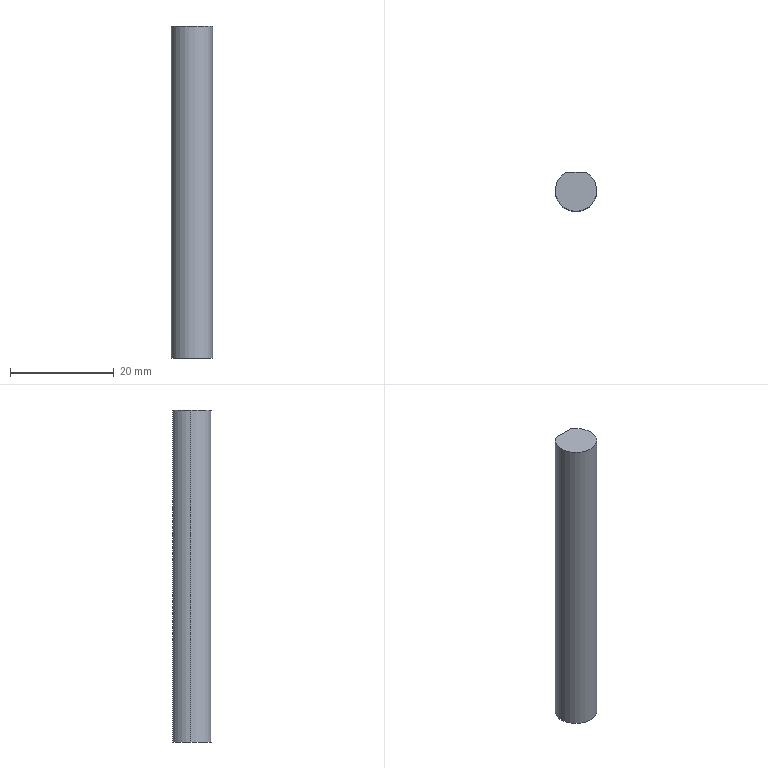Part | NX | features BREP 1 | 1 solid | 6 faces | box 8 x 7.5 x 64 mm | volume 3133 mm3 | cylinder 3 | plane 3 | commonest cylinder face diameters 8 x3
STEP:
#1=CARTESIAN_POINT('',(1.936,3.5,63.));
#2=VERTEX_POINT('',#1);
#3=CARTESIAN_POINT('',(4.,0.,63.));
#4=VERTEX_POINT('',#3);
#5=CARTESIAN_POINT('',(0.,0.,63.));
#6=DIRECTION('',(0.,0.,-1.));
#7=DIRECTION('',(-1.,0.,0.));
#8=AXIS2_PLACEMENT_3D('',#5,#6,#7);
#9=CIRCLE('',#8,4.);
#10=EDGE_CURVE('',#2,#4,#9,.T.);
#11=ORIENTED_EDGE('',*,*,#10,.T.);
#12=CARTESIAN_POINT('',(4.,0.,-1.));
#13=VERTEX_POINT('',#12);
#14=CARTESIAN_POINT('',(4.,0.,63.));
#15=DIRECTION('',(0.,0.,-1.));
#16=VECTOR('',#15,1000.);
#17=LINE('',#14,#16);
#18=EDGE_CURVE('',#4,#13,#17,.T.);
#19=ORIENTED_EDGE('',*,*,#18,.T.);
#20=CARTESIAN_POINT('',(1.936,3.5,-1.));
#21=VERTEX_POINT('',#20);
#22=CARTESIAN_POINT('',(0.,0.,-1.));
#23=DIRECTION('',(0.,0.,1.));
#24=DIRECTION('',(-1.,0.,0.));
#25=AXIS2_PLACEMENT_3D('',#22,#23,#24);
#26=CIRCLE('',#25,4.);
#27=EDGE_CURVE('',#13,#21,#26,.T.);
#28=ORIENTED_EDGE('',*,*,#27,.T.);
#29=CARTESIAN_POINT('',(1.936,3.5,63.));
#30=DIRECTION('',(0.,0.,1.));
#31=VECTOR('',#30,1000.);
#32=LINE('',#29,#31);
#33=EDGE_CURVE('',#21,#2,#32,.T.);
#34=ORIENTED_EDGE('',*,*,#33,.T.);
#35=EDGE_LOOP('',(#11,#19,#28,#34));
#36=FACE_BOUND('',#35,.T.);
#37=CARTESIAN_POINT('',(0.,0.,63.));
#38=DIRECTION('',(0.,0.,-1.));
#39=DIRECTION('',(-1.,0.,0.));
#40=AXIS2_PLACEMENT_3D('',#37,#38,#39);
#41=CYLINDRICAL_SURFACE('',#40,4.);
#42=ADVANCED_FACE('',(#36),#41,.T.);
#43=ORIENTED_EDGE('',*,*,#18,.F.);
#44=CARTESIAN_POINT('',(-4.,0.,63.));
#45=VERTEX_POINT('',#44);
#46=CARTESIAN_POINT('',(0.,0.,63.));
#47=DIRECTION('',(0.,0.,-1.));
#48=DIRECTION('',(-1.,0.,0.));
#49=AXIS2_PLACEMENT_3D('',#46,#47,#48);
#50=CIRCLE('',#49,4.);
#51=EDGE_CURVE('',#4,#45,#50,.T.);
#52=ORIENTED_EDGE('',*,*,#51,.T.);
#53=CARTESIAN_POINT('',(-4.,0.,-1.));
#54=VERTEX_POINT('',#53);
#55=CARTESIAN_POINT('',(-4.,0.,63.));
#56=DIRECTION('',(0.,0.,-1.));
#57=VECTOR('',#56,1000.);
#58=LINE('',#55,#57);
#59=EDGE_CURVE('',#45,#54,#58,.T.);
#60=ORIENTED_EDGE('',*,*,#59,.T.);
#61=CARTESIAN_POINT('',(0.,0.,-1.));
#62=DIRECTION('',(0.,0.,1.));
#63=DIRECTION('',(-1.,0.,0.));
#64=AXIS2_PLACEMENT_3D('',#61,#62,#63);
#65=CIRCLE('',#64,4.);
#66=EDGE_CURVE('',#54,#13,#65,.T.);
#67=ORIENTED_EDGE('',*,*,#66,.T.);
#68=EDGE_LOOP('',(#43,#52,#60,#67));
#69=FACE_BOUND('',#68,.T.);
#70=CARTESIAN_POINT('',(0.,0.,63.));
#71=DIRECTION('',(0.,0.,-1.));
#72=DIRECTION('',(-1.,0.,0.));
#73=AXIS2_PLACEMENT_3D('',#70,#71,#72);
#74=CYLINDRICAL_SURFACE('',#73,4.);
#75=ADVANCED_FACE('',(#69),#74,.T.);
#76=ORIENTED_EDGE('',*,*,#59,.F.);
#77=CARTESIAN_POINT('',(-1.936,3.5,63.));
#78=VERTEX_POINT('',#77);
#79=CARTESIAN_POINT('',(0.,0.,63.));
#80=DIRECTION('',(0.,0.,-1.));
#81=DIRECTION('',(-1.,0.,0.));
#82=AXIS2_PLACEMENT_3D('',#79,#80,#81);
#83=CIRCLE('',#82,4.);
#84=EDGE_CURVE('',#45,#78,#83,.T.);
#85=ORIENTED_EDGE('',*,*,#84,.T.);
#86=CARTESIAN_POINT('',(-1.936,3.5,-1.));
#87=VERTEX_POINT('',#86);
#88=CARTESIAN_POINT('',(-1.936,3.5,63.));
#89=DIRECTION('',(0.,0.,-1.));
#90=VECTOR('',#89,1000.);
#91=LINE('',#88,#90);
#92=EDGE_CURVE('',#78,#87,#91,.T.);
#93=ORIENTED_EDGE('',*,*,#92,.T.);
#94=CARTESIAN_POINT('',(0.,0.,-1.));
#95=DIRECTION('',(0.,0.,1.));
#96=DIRECTION('',(-1.,0.,0.));
#97=AXIS2_PLACEMENT_3D('',#94,#95,#96);
#98=CIRCLE('',#97,4.);
#99=EDGE_CURVE('',#87,#54,#98,.T.);
#100=ORIENTED_EDGE('',*,*,#99,.T.);
#101=EDGE_LOOP('',(#76,#85,#93,#100));
#102=FACE_BOUND('',#101,.T.);
#103=CARTESIAN_POINT('',(0.,0.,63.));
#104=DIRECTION('',(0.,0.,-1.));
#105=DIRECTION('',(-1.,0.,0.));
#106=AXIS2_PLACEMENT_3D('',#103,#104,#105);
#107=CYLINDRICAL_SURFACE('',#106,4.);
#108=ADVANCED_FACE('',(#102),#107,.T.);
#109=CARTESIAN_POINT('',(0.,3.5,-1.));
#110=DIRECTION('',(-1.,0.,0.));
#111=VECTOR('',#110,1000.);
#112=LINE('',#109,#111);
#113=EDGE_CURVE('',#21,#87,#112,.T.);
#114=ORIENTED_EDGE('',*,*,#113,.F.);
#115=ORIENTED_EDGE('',*,*,#27,.F.);
#116=ORIENTED_EDGE('',*,*,#66,.F.);
#117=ORIENTED_EDGE('',*,*,#99,.F.);
#118=EDGE_LOOP('',(#114,#115,#116,#117));
#119=FACE_BOUND('',#118,.T.);
#120=CARTESIAN_POINT('',(0.,0.,-1.));
#121=DIRECTION('',(0.,0.,1.));
#122=DIRECTION('',(1.,0.,0.));
#123=AXIS2_PLACEMENT_3D('',#120,#121,#122);
#124=PLANE('',#123);
#125=ADVANCED_FACE('',(#119),#124,.F.);
#126=ORIENTED_EDGE('',*,*,#10,.F.);
#127=CARTESIAN_POINT('',(0.,3.5,63.));
#128=DIRECTION('',(-1.,0.,0.));
#129=VECTOR('',#128,1000.);
#130=LINE('',#127,#129);
#131=EDGE_CURVE('',#2,#78,#130,.T.);
#132=ORIENTED_EDGE('',*,*,#131,.T.);
#133=ORIENTED_EDGE('',*,*,#84,.F.);
#134=ORIENTED_EDGE('',*,*,#51,.F.);
#135=EDGE_LOOP('',(#126,#132,#133,#134));
#136=FACE_BOUND('',#135,.T.);
#137=CARTESIAN_POINT('',(0.,0.,63.));
#138=DIRECTION('',(0.,0.,1.));
#139=DIRECTION('',(1.,0.,0.));
#140=AXIS2_PLACEMENT_3D('',#137,#138,#139);
#141=PLANE('',#140);
#142=ADVANCED_FACE('',(#136),#141,.T.);
#143=ORIENTED_EDGE('',*,*,#92,.F.);
#144=ORIENTED_EDGE('',*,*,#131,.F.);
#145=ORIENTED_EDGE('',*,*,#33,.F.);
#146=ORIENTED_EDGE('',*,*,#113,.T.);
#147=EDGE_LOOP('',(#143,#144,#145,#146));
#148=FACE_BOUND('',#147,.T.);
#149=CARTESIAN_POINT('',(7.783,3.5,63.));
#150=DIRECTION('',(0.,1.,0.));
#151=DIRECTION('',(1.,0.,0.));
#152=AXIS2_PLACEMENT_3D('',#149,#150,#151);
#153=PLANE('',#152);
#154=ADVANCED_FACE('',(#148),#153,.T.);
#155=CLOSED_SHELL('',(#42,#75,#108,#125,#142,#154));
#156=MANIFOLD_SOLID_BREP('',#155);
#157=(LENGTH_UNIT()NAMED_UNIT(*)SI_UNIT(.MILLI.,.METRE.));
#158=UNCERTAINTY_MEASURE_WITH_UNIT(LENGTH_MEASURE(0.00001),#157,'','');
#159=(NAMED_UNIT(*)PLANE_ANGLE_UNIT()SI_UNIT($,.RADIAN.));
#160=(NAMED_UNIT(*)SI_UNIT($,.STERADIAN.)SOLID_ANGLE_UNIT());
#161=(GEOMETRIC_REPRESENTATION_CONTEXT(3)GLOBAL_UNCERTAINTY_ASSIGNED_CONTEXT((#158))GLOBAL_UNIT_ASSIGNED_CONTEXT((#157,#159,#160))REPRESENTATION_CONTEXT('',''));
#162=ADVANCED_BREP_SHAPE_REPRESENTATION('',(#156),#161);